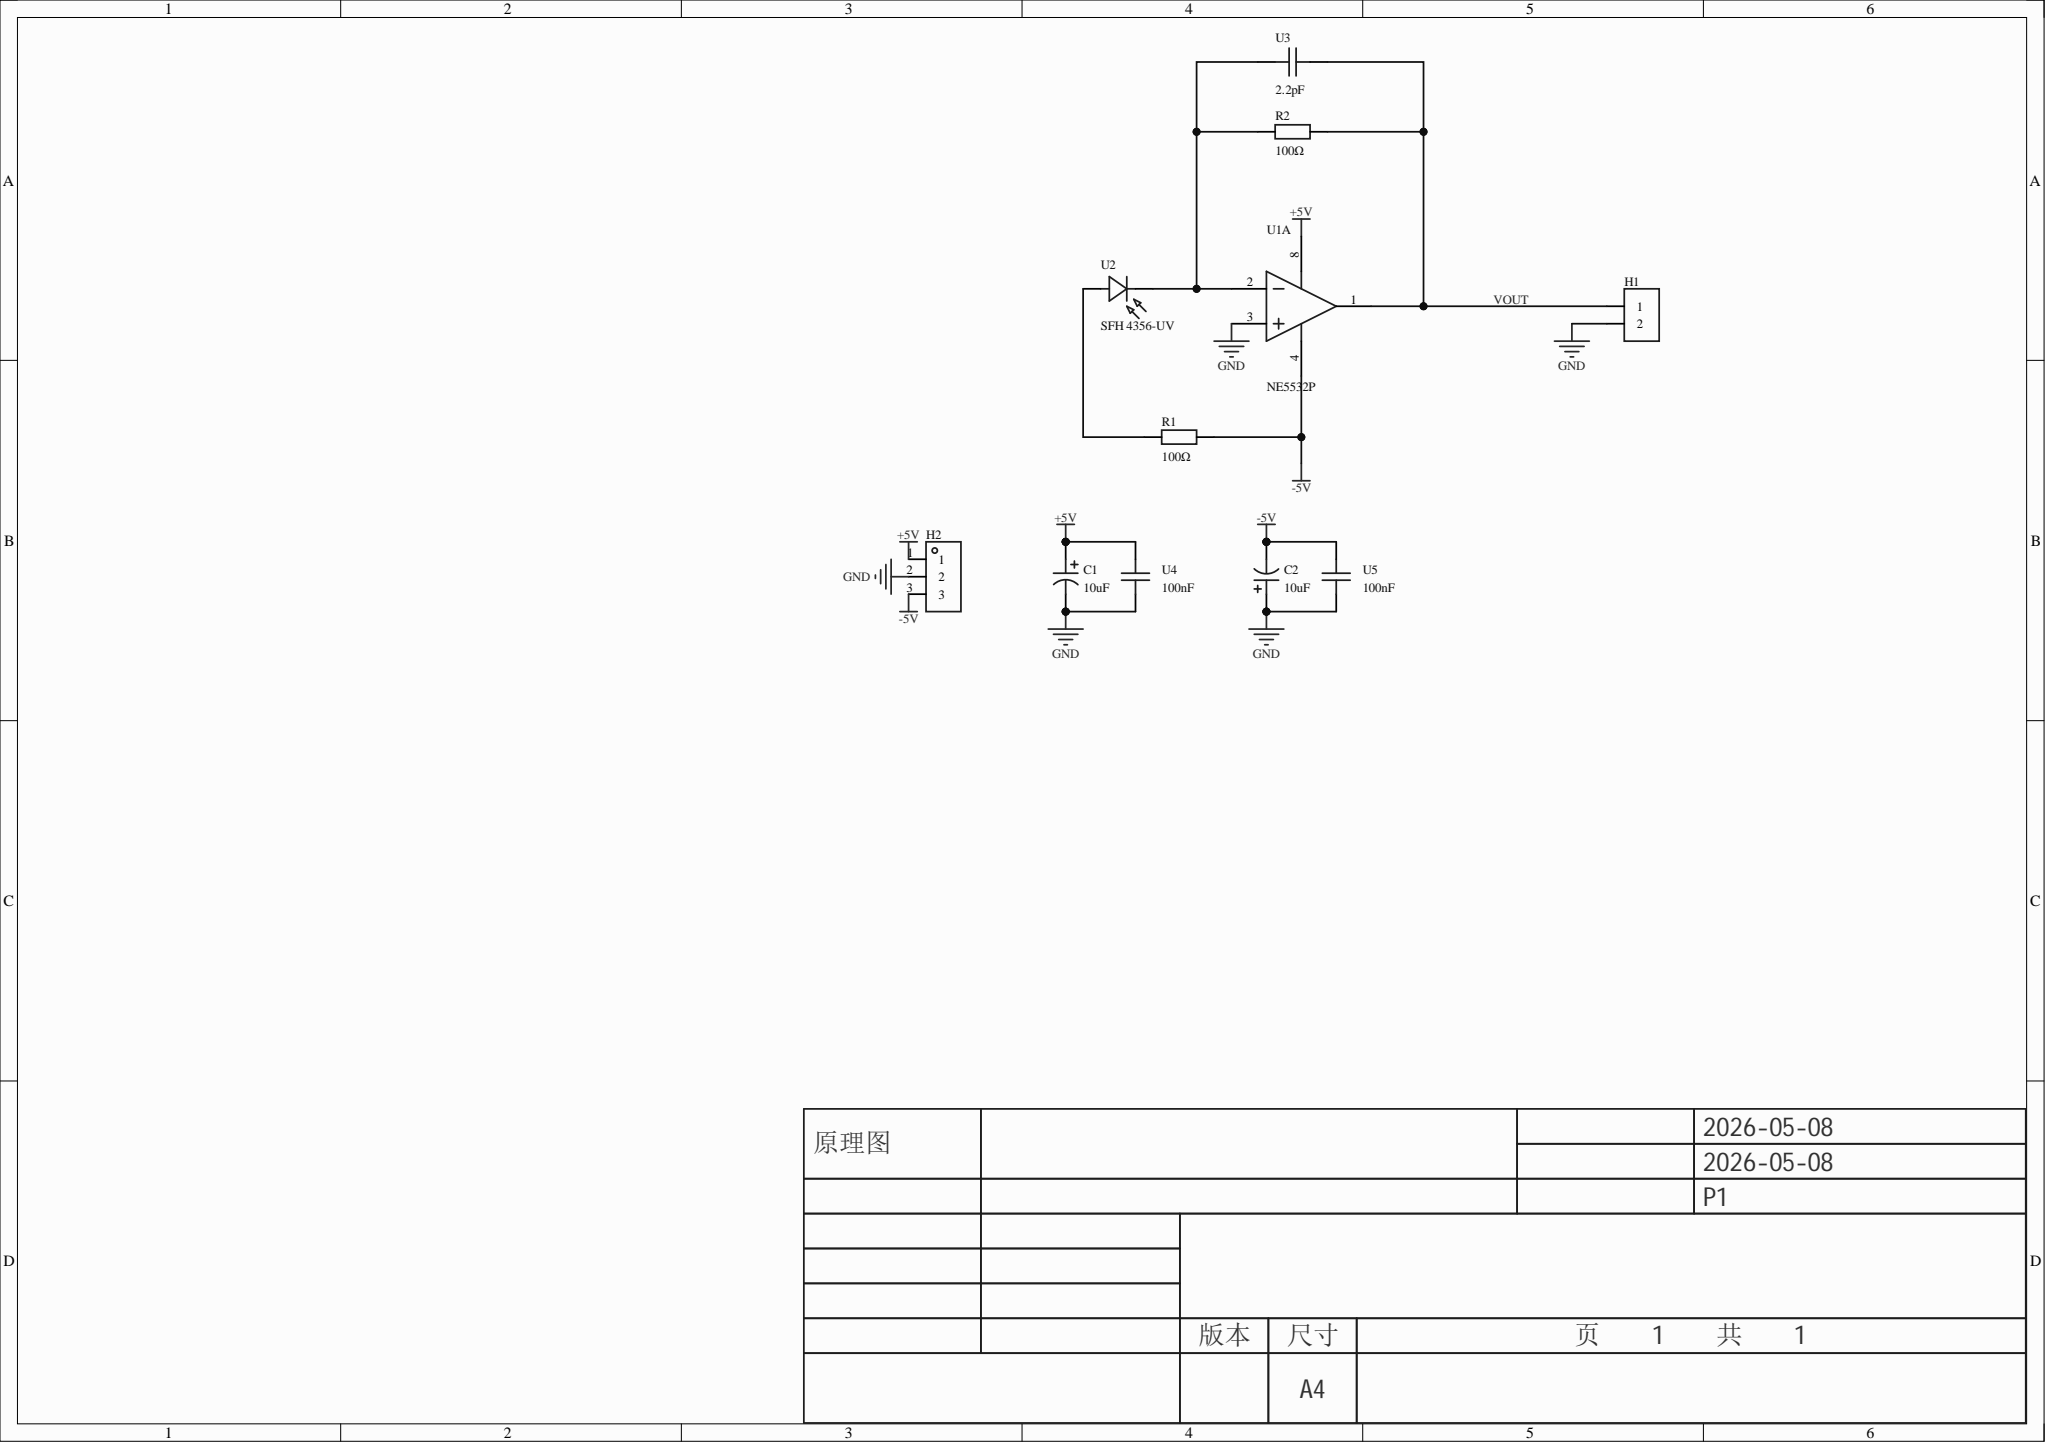Circuit board | Altium Designer | 11 parts | 6 nets
Bill of materials:
Comment,Description,Designator,Footprint,LibRef,Quantity
"10uF","","C1, C2","CAP-TH_BD5.0-P2.00-D0.8-FD-10UF50VC110GL","10UF50VC110GL","2"
"","","H1","HDR-TH_2P-P2.54-V-F","HDR-F_2.54_1x2P","1"
"","","H2","HDR-TH_3P-P2.54-V-F","HDR-F_2.54_1x3P","1"
"100Ω","","R1, R2","Res_1/8W","Res_AXIAL-1/8W","2"
"NE5532P","放大器数:2;轨到轨:-;增益带宽积(GBW):10MHz;输入失调电压(Vos):4mV;压摆率(SR):9V/us;输入偏置电流(Ib):1uA;","U1","DIP-8_L9.4-W6.4-P2.54-LS9.1-BL","NE5532P","1"
"SFH 4356-UV","正向电压:1.7V;波长:860nm;辐射强度:40mW/sr@100mA;视角:40°;","U2","LED-TH_BD3.8-P2.54-FD","SFH 4356-UV","1"
"2.2pF","","U3","CAP-TH_L5.0-W2.5-P5.00-D1.0","100nF","1"
"100nF","","U4, U5","CAP-TH_L5.0-W2.5-P5.00-D1.0","100nF","2"
Netlist (Protel format):
[
C1
CAP-TH_BD5.0-P2.00-D0.8-FD-10UF50VC110GL
10uF



]
[
C2
CAP-TH_BD5.0-P2.00-D0.8-FD-10UF50VC110GL
10uF



]
[
H1
HDR-TH_2P-P2.54-V-F




]
[
H2
HDR-TH_3P-P2.54-V-F




]
[
R1
Res_1/8W
100Ω



]
[
R2
Res_1/8W
100Ω



]
[
U1
DIP-8_L9.4-W6.4-P2.54-LS9.1-BL
NE5532P



]
[
U2
LED-TH_BD3.8-P2.54-FD
SFH 4356-UV



]
[
U3
CAP-TH_L5.0-W2.5-P5.00-D1.0
2.2pF



]
[
U4
CAP-TH_L5.0-W2.5-P5.00-D1.0
100nF



]
[
U5
CAP-TH_L5.0-W2.5-P5.00-D1.0
100nF



]
(
VOUT
H1-1
R2-2
U1-1
U3-1
)
(
NetR2_1
R2-1
U1-2
U2-2
U3-2
)
(
NetR1_1
R1-1
U2-1
)
(
GND
C1-2
C2-1
H1-2
H2-2
U1-3
U4-2
U5-2
)
(
-5V
C2-2
H2-3
R1-2
U1-4
U5-1
)
(
+5V
C1-1
H2-1
U1-8
U4-1
)